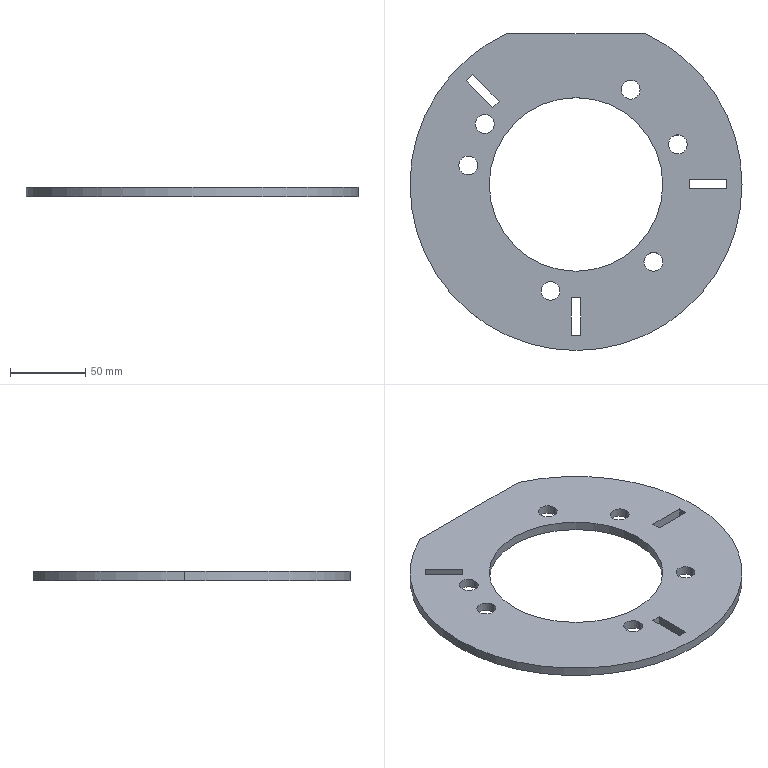Part | SolidWorks | features FlatPattern 1, SMBaseFlange 1, SheetMetal 1 | 1 solid | 32 faces | box 220 x 210 x 6 mm | volume 154940 mm3 | cylinder 17 | plane 15 | commonest cylinder face diameters 12.5 x12 220 x3 115 x2
STEP:
#1=CARTESIAN_POINT('',(92.731,46.962,6.));
#2=VERTEX_POINT('',#1);
#3=CARTESIAN_POINT('',(105.231,46.962,6.));
#4=VERTEX_POINT('',#3);
#5=CARTESIAN_POINT('',(98.981,46.962,6.));
#6=DIRECTION('',(0.,0.,1.));
#7=DIRECTION('',(1.,0.,0.));
#8=AXIS2_PLACEMENT_3D('',#5,#6,#7);
#9=CIRCLE('',#8,6.25);
#10=EDGE_CURVE('',#2,#4,#9,.T.);
#11=ORIENTED_EDGE('',*,*,#10,.T.);
#12=CARTESIAN_POINT('',(105.231,46.962,0.));
#13=VERTEX_POINT('',#12);
#14=CARTESIAN_POINT('',(105.231,46.962,6.));
#15=DIRECTION('',(0.,0.,-1.));
#16=VECTOR('',#15,1000.);
#17=LINE('',#14,#16);
#18=EDGE_CURVE('',#4,#13,#17,.T.);
#19=ORIENTED_EDGE('',*,*,#18,.T.);
#20=CARTESIAN_POINT('',(92.731,46.962,0.));
#21=VERTEX_POINT('',#20);
#22=CARTESIAN_POINT('',(98.981,46.962,0.));
#23=DIRECTION('',(0.,0.,1.));
#24=DIRECTION('',(1.,0.,0.));
#25=AXIS2_PLACEMENT_3D('',#22,#23,#24);
#26=CIRCLE('',#25,6.25);
#27=EDGE_CURVE('',#21,#13,#26,.T.);
#28=ORIENTED_EDGE('',*,*,#27,.F.);
#29=CARTESIAN_POINT('',(92.731,46.962,6.));
#30=DIRECTION('',(0.,0.,-1.));
#31=VECTOR('',#30,1000.);
#32=LINE('',#29,#31);
#33=EDGE_CURVE('',#2,#21,#32,.T.);
#34=ORIENTED_EDGE('',*,*,#33,.F.);
#35=EDGE_LOOP('',(#11,#19,#28,#34));
#36=FACE_OUTER_BOUND('',#35,.T.);
#37=CARTESIAN_POINT('',(98.981,46.962,6.));
#38=DIRECTION('',(0.,0.,-1.));
#39=DIRECTION('',(-1.,0.,0.));
#40=AXIS2_PLACEMENT_3D('',#37,#38,#39);
#41=CYLINDRICAL_SURFACE('',#40,6.25);
#42=ADVANCED_FACE('',(#36),#41,.F.);
#43=CARTESIAN_POINT('',(-3.976,24.191,6.));
#44=VERTEX_POINT('',#43);
#45=CARTESIAN_POINT('',(8.524,24.191,6.));
#46=VERTEX_POINT('',#45);
#47=CARTESIAN_POINT('',(2.274,24.191,6.));
#48=DIRECTION('',(0.,0.,1.));
#49=DIRECTION('',(1.,0.,0.));
#50=AXIS2_PLACEMENT_3D('',#47,#48,#49);
#51=CIRCLE('',#50,6.25);
#52=EDGE_CURVE('',#44,#46,#51,.T.);
#53=ORIENTED_EDGE('',*,*,#52,.T.);
#54=CARTESIAN_POINT('',(8.524,24.191,0.));
#55=VERTEX_POINT('',#54);
#56=CARTESIAN_POINT('',(8.524,24.191,6.));
#57=DIRECTION('',(0.,0.,-1.));
#58=VECTOR('',#57,1000.);
#59=LINE('',#56,#58);
#60=EDGE_CURVE('',#46,#55,#59,.T.);
#61=ORIENTED_EDGE('',*,*,#60,.T.);
#62=CARTESIAN_POINT('',(-3.976,24.191,0.));
#63=VERTEX_POINT('',#62);
#64=CARTESIAN_POINT('',(2.274,24.191,0.));
#65=DIRECTION('',(0.,0.,1.));
#66=DIRECTION('',(1.,0.,0.));
#67=AXIS2_PLACEMENT_3D('',#64,#65,#66);
#68=CIRCLE('',#67,6.25);
#69=EDGE_CURVE('',#63,#55,#68,.T.);
#70=ORIENTED_EDGE('',*,*,#69,.F.);
#71=CARTESIAN_POINT('',(-3.976,24.191,6.));
#72=DIRECTION('',(0.,0.,-1.));
#73=VECTOR('',#72,1000.);
#74=LINE('',#71,#73);
#75=EDGE_CURVE('',#44,#63,#74,.T.);
#76=ORIENTED_EDGE('',*,*,#75,.F.);
#77=EDGE_LOOP('',(#53,#61,#70,#76));
#78=FACE_OUTER_BOUND('',#77,.T.);
#79=CARTESIAN_POINT('',(2.274,24.191,6.));
#80=DIRECTION('',(0.,0.,-1.));
#81=DIRECTION('',(-1.,0.,0.));
#82=AXIS2_PLACEMENT_3D('',#79,#80,#81);
#83=CYLINDRICAL_SURFACE('',#82,6.25);
#84=ADVANCED_FACE('',(#78),#83,.F.);
#85=CARTESIAN_POINT('',(-14.918,-3.235,6.));
#86=VERTEX_POINT('',#85);
#87=CARTESIAN_POINT('',(-2.418,-3.235,6.));
#88=VERTEX_POINT('',#87);
#89=CARTESIAN_POINT('',(-8.668,-3.235,6.));
#90=DIRECTION('',(0.,0.,1.));
#91=DIRECTION('',(1.,0.,0.));
#92=AXIS2_PLACEMENT_3D('',#89,#90,#91);
#93=CIRCLE('',#92,6.25);
#94=EDGE_CURVE('',#86,#88,#93,.T.);
#95=ORIENTED_EDGE('',*,*,#94,.T.);
#96=CARTESIAN_POINT('',(-2.418,-3.235,0.));
#97=VERTEX_POINT('',#96);
#98=CARTESIAN_POINT('',(-2.418,-3.235,6.));
#99=DIRECTION('',(0.,0.,-1.));
#100=VECTOR('',#99,1000.);
#101=LINE('',#98,#100);
#102=EDGE_CURVE('',#88,#97,#101,.T.);
#103=ORIENTED_EDGE('',*,*,#102,.T.);
#104=CARTESIAN_POINT('',(-14.918,-3.235,0.));
#105=VERTEX_POINT('',#104);
#106=CARTESIAN_POINT('',(-8.668,-3.235,0.));
#107=DIRECTION('',(0.,0.,1.));
#108=DIRECTION('',(1.,0.,0.));
#109=AXIS2_PLACEMENT_3D('',#106,#107,#108);
#110=CIRCLE('',#109,6.25);
#111=EDGE_CURVE('',#105,#97,#110,.T.);
#112=ORIENTED_EDGE('',*,*,#111,.F.);
#113=CARTESIAN_POINT('',(-14.918,-3.235,6.));
#114=DIRECTION('',(0.,0.,-1.));
#115=VECTOR('',#114,1000.);
#116=LINE('',#113,#115);
#117=EDGE_CURVE('',#86,#105,#116,.T.);
#118=ORIENTED_EDGE('',*,*,#117,.F.);
#119=EDGE_LOOP('',(#95,#103,#112,#118));
#120=FACE_OUTER_BOUND('',#119,.T.);
#121=CARTESIAN_POINT('',(-8.668,-3.235,6.));
#122=DIRECTION('',(0.,0.,-1.));
#123=DIRECTION('',(-1.,0.,0.));
#124=AXIS2_PLACEMENT_3D('',#121,#122,#123);
#125=CYLINDRICAL_SURFACE('',#124,6.25);
#126=ADVANCED_FACE('',(#120),#125,.F.);
#127=CARTESIAN_POINT('',(39.556,-86.321,6.));
#128=VERTEX_POINT('',#127);
#129=CARTESIAN_POINT('',(52.056,-86.321,6.));
#130=VERTEX_POINT('',#129);
#131=CARTESIAN_POINT('',(45.806,-86.321,6.));
#132=DIRECTION('',(0.,0.,1.));
#133=DIRECTION('',(1.,0.,0.));
#134=AXIS2_PLACEMENT_3D('',#131,#132,#133);
#135=CIRCLE('',#134,6.25);
#136=EDGE_CURVE('',#128,#130,#135,.T.);
#137=ORIENTED_EDGE('',*,*,#136,.T.);
#138=CARTESIAN_POINT('',(52.056,-86.321,0.));
#139=VERTEX_POINT('',#138);
#140=CARTESIAN_POINT('',(52.056,-86.321,6.));
#141=DIRECTION('',(0.,0.,-1.));
#142=VECTOR('',#141,1000.);
#143=LINE('',#140,#142);
#144=EDGE_CURVE('',#130,#139,#143,.T.);
#145=ORIENTED_EDGE('',*,*,#144,.T.);
#146=CARTESIAN_POINT('',(39.556,-86.321,0.));
#147=VERTEX_POINT('',#146);
#148=CARTESIAN_POINT('',(45.806,-86.321,0.));
#149=DIRECTION('',(0.,0.,1.));
#150=DIRECTION('',(1.,0.,0.));
#151=AXIS2_PLACEMENT_3D('',#148,#149,#150);
#152=CIRCLE('',#151,6.25);
#153=EDGE_CURVE('',#147,#139,#152,.T.);
#154=ORIENTED_EDGE('',*,*,#153,.F.);
#155=CARTESIAN_POINT('',(39.556,-86.321,6.));
#156=DIRECTION('',(0.,0.,-1.));
#157=VECTOR('',#156,1000.);
#158=LINE('',#155,#157);
#159=EDGE_CURVE('',#128,#147,#158,.T.);
#160=ORIENTED_EDGE('',*,*,#159,.F.);
#161=EDGE_LOOP('',(#137,#145,#154,#160));
#162=FACE_OUTER_BOUND('',#161,.T.);
#163=CARTESIAN_POINT('',(45.806,-86.321,6.));
#164=DIRECTION('',(0.,0.,-1.));
#165=DIRECTION('',(-1.,0.,0.));
#166=AXIS2_PLACEMENT_3D('',#163,#164,#165);
#167=CYLINDRICAL_SURFACE('',#166,6.25);
#168=ADVANCED_FACE('',(#162),#167,.F.);
#169=CARTESIAN_POINT('',(107.746,-67.09,6.));
#170=VERTEX_POINT('',#169);
#171=CARTESIAN_POINT('',(120.246,-67.09,6.));
#172=VERTEX_POINT('',#171);
#173=CARTESIAN_POINT('',(113.996,-67.09,6.));
#174=DIRECTION('',(0.,0.,1.));
#175=DIRECTION('',(1.,0.,0.));
#176=AXIS2_PLACEMENT_3D('',#173,#174,#175);
#177=CIRCLE('',#176,6.25);
#178=EDGE_CURVE('',#170,#172,#177,.T.);
#179=ORIENTED_EDGE('',*,*,#178,.T.);
#180=CARTESIAN_POINT('',(120.246,-67.09,0.));
#181=VERTEX_POINT('',#180);
#182=CARTESIAN_POINT('',(120.246,-67.09,6.));
#183=DIRECTION('',(0.,0.,-1.));
#184=VECTOR('',#183,1000.);
#185=LINE('',#182,#184);
#186=EDGE_CURVE('',#172,#181,#185,.T.);
#187=ORIENTED_EDGE('',*,*,#186,.T.);
#188=CARTESIAN_POINT('',(107.746,-67.09,0.));
#189=VERTEX_POINT('',#188);
#190=CARTESIAN_POINT('',(113.996,-67.09,0.));
#191=DIRECTION('',(0.,0.,1.));
#192=DIRECTION('',(1.,0.,0.));
#193=AXIS2_PLACEMENT_3D('',#190,#191,#192);
#194=CIRCLE('',#193,6.25);
#195=EDGE_CURVE('',#189,#181,#194,.T.);
#196=ORIENTED_EDGE('',*,*,#195,.F.);
#197=CARTESIAN_POINT('',(107.746,-67.09,6.));
#198=DIRECTION('',(0.,0.,-1.));
#199=VECTOR('',#198,1000.);
#200=LINE('',#197,#199);
#201=EDGE_CURVE('',#170,#189,#200,.T.);
#202=ORIENTED_EDGE('',*,*,#201,.F.);
#203=EDGE_LOOP('',(#179,#187,#196,#202));
#204=FACE_OUTER_BOUND('',#203,.T.);
#205=CARTESIAN_POINT('',(113.996,-67.09,6.));
#206=DIRECTION('',(0.,0.,-1.));
#207=DIRECTION('',(-1.,0.,0.));
#208=AXIS2_PLACEMENT_3D('',#205,#206,#207);
#209=CYLINDRICAL_SURFACE('',#208,6.25);
#210=ADVANCED_FACE('',(#204),#209,.F.);
#211=CARTESIAN_POINT('',(123.936,10.747,6.));
#212=VERTEX_POINT('',#211);
#213=CARTESIAN_POINT('',(136.436,10.747,6.));
#214=VERTEX_POINT('',#213);
#215=CARTESIAN_POINT('',(130.186,10.747,6.));
#216=DIRECTION('',(0.,0.,1.));
#217=DIRECTION('',(1.,0.,0.));
#218=AXIS2_PLACEMENT_3D('',#215,#216,#217);
#219=CIRCLE('',#218,6.25);
#220=EDGE_CURVE('',#212,#214,#219,.T.);
#221=ORIENTED_EDGE('',*,*,#220,.T.);
#222=CARTESIAN_POINT('',(136.436,10.747,0.));
#223=VERTEX_POINT('',#222);
#224=CARTESIAN_POINT('',(136.436,10.747,6.));
#225=DIRECTION('',(0.,0.,-1.));
#226=VECTOR('',#225,1000.);
#227=LINE('',#224,#226);
#228=EDGE_CURVE('',#214,#223,#227,.T.);
#229=ORIENTED_EDGE('',*,*,#228,.T.);
#230=CARTESIAN_POINT('',(123.936,10.747,0.));
#231=VERTEX_POINT('',#230);
#232=CARTESIAN_POINT('',(130.186,10.747,0.));
#233=DIRECTION('',(0.,0.,1.));
#234=DIRECTION('',(1.,0.,0.));
#235=AXIS2_PLACEMENT_3D('',#232,#233,#234);
#236=CIRCLE('',#235,6.25);
#237=EDGE_CURVE('',#231,#223,#236,.T.);
#238=ORIENTED_EDGE('',*,*,#237,.F.);
#239=CARTESIAN_POINT('',(123.936,10.747,6.));
#240=DIRECTION('',(0.,0.,-1.));
#241=VECTOR('',#240,1000.);
#242=LINE('',#239,#241);
#243=EDGE_CURVE('',#212,#231,#242,.T.);
#244=ORIENTED_EDGE('',*,*,#243,.F.);
#245=EDGE_LOOP('',(#221,#229,#238,#244));
#246=FACE_OUTER_BOUND('',#245,.T.);
#247=CARTESIAN_POINT('',(130.186,10.747,6.));
#248=DIRECTION('',(0.,0.,-1.));
#249=DIRECTION('',(-1.,0.,0.));
#250=AXIS2_PLACEMENT_3D('',#247,#248,#249);
#251=CYLINDRICAL_SURFACE('',#250,6.25);
#252=ADVANCED_FACE('',(#246),#251,.F.);
#253=CARTESIAN_POINT('',(5.231,-15.825,6.));
#254=VERTEX_POINT('',#253);
#255=CARTESIAN_POINT('',(120.231,-15.825,6.));
#256=VERTEX_POINT('',#255);
#257=CARTESIAN_POINT('',(62.731,-15.825,6.));
#258=DIRECTION('',(0.,0.,1.));
#259=DIRECTION('',(1.,0.,0.));
#260=AXIS2_PLACEMENT_3D('',#257,#258,#259);
#261=CIRCLE('',#260,57.5);
#262=EDGE_CURVE('',#254,#256,#261,.T.);
#263=ORIENTED_EDGE('',*,*,#262,.T.);
#264=CARTESIAN_POINT('',(120.231,-15.825,0.));
#265=VERTEX_POINT('',#264);
#266=CARTESIAN_POINT('',(120.231,-15.825,6.));
#267=DIRECTION('',(0.,0.,-1.));
#268=VECTOR('',#267,1000.);
#269=LINE('',#266,#268);
#270=EDGE_CURVE('',#256,#265,#269,.T.);
#271=ORIENTED_EDGE('',*,*,#270,.T.);
#272=CARTESIAN_POINT('',(5.231,-15.825,0.));
#273=VERTEX_POINT('',#272);
#274=CARTESIAN_POINT('',(62.731,-15.825,0.));
#275=DIRECTION('',(0.,0.,1.));
#276=DIRECTION('',(1.,0.,0.));
#277=AXIS2_PLACEMENT_3D('',#274,#275,#276);
#278=CIRCLE('',#277,57.5);
#279=EDGE_CURVE('',#273,#265,#278,.T.);
#280=ORIENTED_EDGE('',*,*,#279,.F.);
#281=CARTESIAN_POINT('',(5.231,-15.825,6.));
#282=DIRECTION('',(0.,0.,-1.));
#283=VECTOR('',#282,1000.);
#284=LINE('',#281,#283);
#285=EDGE_CURVE('',#254,#273,#284,.T.);
#286=ORIENTED_EDGE('',*,*,#285,.F.);
#287=EDGE_LOOP('',(#263,#271,#280,#286));
#288=FACE_OUTER_BOUND('',#287,.T.);
#289=CARTESIAN_POINT('',(62.731,-15.825,6.));
#290=DIRECTION('',(0.,0.,-1.));
#291=DIRECTION('',(-1.,0.,0.));
#292=AXIS2_PLACEMENT_3D('',#289,#290,#291);
#293=CYLINDRICAL_SURFACE('',#292,57.5);
#294=ADVANCED_FACE('',(#288),#293,.F.);
#295=CARTESIAN_POINT('',(172.731,-15.825,6.));
#296=VERTEX_POINT('',#295);
#297=CARTESIAN_POINT('',(108.557,84.175,6.));
#298=VERTEX_POINT('',#297);
#299=CARTESIAN_POINT('',(62.731,-15.825,6.));
#300=DIRECTION('',(0.,0.,1.));
#301=DIRECTION('',(1.,0.,0.));
#302=AXIS2_PLACEMENT_3D('',#299,#300,#301);
#303=CIRCLE('',#302,110.);
#304=EDGE_CURVE('',#296,#298,#303,.T.);
#305=ORIENTED_EDGE('',*,*,#304,.F.);
#306=CARTESIAN_POINT('',(172.731,-15.825,0.));
#307=VERTEX_POINT('',#306);
#308=CARTESIAN_POINT('',(172.731,-15.825,6.));
#309=DIRECTION('',(0.,0.,-1.));
#310=VECTOR('',#309,1000.);
#311=LINE('',#308,#310);
#312=EDGE_CURVE('',#296,#307,#311,.T.);
#313=ORIENTED_EDGE('',*,*,#312,.T.);
#314=CARTESIAN_POINT('',(108.557,84.175,0.));
#315=VERTEX_POINT('',#314);
#316=CARTESIAN_POINT('',(62.731,-15.825,0.));
#317=DIRECTION('',(0.,0.,1.));
#318=DIRECTION('',(1.,0.,0.));
#319=AXIS2_PLACEMENT_3D('',#316,#317,#318);
#320=CIRCLE('',#319,110.);
#321=EDGE_CURVE('',#307,#315,#320,.T.);
#322=ORIENTED_EDGE('',*,*,#321,.T.);
#323=CARTESIAN_POINT('',(108.557,84.175,6.));
#324=DIRECTION('',(0.,0.,-1.));
#325=VECTOR('',#324,1000.);
#326=LINE('',#323,#325);
#327=EDGE_CURVE('',#298,#315,#326,.T.);
#328=ORIENTED_EDGE('',*,*,#327,.F.);
#329=EDGE_LOOP('',(#305,#313,#322,#328));
#330=FACE_OUTER_BOUND('',#329,.T.);
#331=CARTESIAN_POINT('',(62.731,-15.825,6.));
#332=DIRECTION('',(0.,0.,-1.));
#333=DIRECTION('',(-1.,0.,0.));
#334=AXIS2_PLACEMENT_3D('',#331,#332,#333);
#335=CYLINDRICAL_SURFACE('',#334,110.);
#336=ADVANCED_FACE('',(#330),#335,.T.);
#337=ORIENTED_EDGE('',*,*,#312,.F.);
#338=CARTESIAN_POINT('',(-47.269,-15.825,6.));
#339=VERTEX_POINT('',#338);
#340=CARTESIAN_POINT('',(62.731,-15.825,6.));
#341=DIRECTION('',(0.,0.,1.));
#342=DIRECTION('',(1.,0.,0.));
#343=AXIS2_PLACEMENT_3D('',#340,#341,#342);
#344=CIRCLE('',#343,110.);
#345=EDGE_CURVE('',#339,#296,#344,.T.);
#346=ORIENTED_EDGE('',*,*,#345,.F.);
#347=CARTESIAN_POINT('',(-47.269,-15.825,0.));
#348=VERTEX_POINT('',#347);
#349=CARTESIAN_POINT('',(-47.269,-15.825,6.));
#350=DIRECTION('',(0.,0.,-1.));
#351=VECTOR('',#350,1000.);
#352=LINE('',#349,#351);
#353=EDGE_CURVE('',#339,#348,#352,.T.);
#354=ORIENTED_EDGE('',*,*,#353,.T.);
#355=CARTESIAN_POINT('',(62.731,-15.825,0.));
#356=DIRECTION('',(0.,0.,1.));
#357=DIRECTION('',(1.,0.,0.));
#358=AXIS2_PLACEMENT_3D('',#355,#356,#357);
#359=CIRCLE('',#358,110.);
#360=EDGE_CURVE('',#348,#307,#359,.T.);
#361=ORIENTED_EDGE('',*,*,#360,.T.);
#362=EDGE_LOOP('',(#337,#346,#354,#361));
#363=FACE_OUTER_BOUND('',#362,.T.);
#364=CARTESIAN_POINT('',(62.731,-15.825,6.));
#365=DIRECTION('',(0.,0.,-1.));
#366=DIRECTION('',(-1.,0.,0.));
#367=AXIS2_PLACEMENT_3D('',#364,#365,#366);
#368=CYLINDRICAL_SURFACE('',#367,110.);
#369=ADVANCED_FACE('',(#363),#368,.T.);
#370=ORIENTED_EDGE('',*,*,#52,.F.);
#371=CARTESIAN_POINT('',(2.274,24.191,6.));
#372=DIRECTION('',(0.,0.,1.));
#373=DIRECTION('',(1.,0.,0.));
#374=AXIS2_PLACEMENT_3D('',#371,#372,#373);
#375=CIRCLE('',#374,6.25);
#376=EDGE_CURVE('',#46,#44,#375,.T.);
#377=ORIENTED_EDGE('',*,*,#376,.F.);
#378=EDGE_LOOP('',(#370,#377));
#379=FACE_BOUND('',#378,.T.);
#380=ORIENTED_EDGE('',*,*,#136,.F.);
#381=CARTESIAN_POINT('',(45.806,-86.321,6.));
#382=DIRECTION('',(0.,0.,1.));
#383=DIRECTION('',(1.,0.,0.));
#384=AXIS2_PLACEMENT_3D('',#381,#382,#383);
#385=CIRCLE('',#384,6.25);
#386=EDGE_CURVE('',#130,#128,#385,.T.);
#387=ORIENTED_EDGE('',*,*,#386,.F.);
#388=EDGE_LOOP('',(#380,#387));
#389=FACE_BOUND('',#388,.T.);
#390=ORIENTED_EDGE('',*,*,#220,.F.);
#391=CARTESIAN_POINT('',(130.186,10.747,6.));
#392=DIRECTION('',(0.,0.,1.));
#393=DIRECTION('',(1.,0.,0.));
#394=AXIS2_PLACEMENT_3D('',#391,#392,#393);
#395=CIRCLE('',#394,6.25);
#396=EDGE_CURVE('',#214,#212,#395,.T.);
#397=ORIENTED_EDGE('',*,*,#396,.F.);
#398=EDGE_LOOP('',(#390,#397));
#399=FACE_BOUND('',#398,.T.);
#400=CARTESIAN_POINT('',(16.905,84.175,6.));
#401=VERTEX_POINT('',#400);
#402=CARTESIAN_POINT('',(62.731,-15.825,6.));
#403=DIRECTION('',(0.,0.,1.));
#404=DIRECTION('',(1.,0.,0.));
#405=AXIS2_PLACEMENT_3D('',#402,#403,#404);
#406=CIRCLE('',#405,110.);
#407=EDGE_CURVE('',#401,#339,#406,.T.);
#408=ORIENTED_EDGE('',*,*,#407,.T.);
#409=ORIENTED_EDGE('',*,*,#345,.T.);
#410=ORIENTED_EDGE('',*,*,#304,.T.);
#411=CARTESIAN_POINT('',(16.905,84.175,6.));
#412=DIRECTION('',(-1.,0.,0.));
#413=VECTOR('',#412,1000.);
#414=LINE('',#411,#413);
#415=EDGE_CURVE('',#298,#401,#414,.T.);
#416=ORIENTED_EDGE('',*,*,#415,.T.);
#417=EDGE_LOOP('',(#408,#409,#410,#416));
#418=FACE_OUTER_BOUND('',#417,.T.);
#419=ORIENTED_EDGE('',*,*,#262,.F.);
#420=CARTESIAN_POINT('',(62.731,-15.825,6.));
#421=DIRECTION('',(0.,0.,1.));
#422=DIRECTION('',(1.,0.,0.));
#423=AXIS2_PLACEMENT_3D('',#420,#421,#422);
#424=CIRCLE('',#423,57.5);
#425=EDGE_CURVE('',#256,#254,#424,.T.);
#426=ORIENTED_EDGE('',*,*,#425,.F.);
#427=EDGE_LOOP('',(#419,#426));
#428=FACE_BOUND('',#427,.T.);
#429=ORIENTED_EDGE('',*,*,#178,.F.);
#430=CARTESIAN_POINT('',(113.996,-67.09,6.));
#431=DIRECTION('',(0.,0.,1.));
#432=DIRECTION('',(1.,0.,0.));
#433=AXIS2_PLACEMENT_3D('',#430,#431,#432);
#434=CIRCLE('',#433,6.25);
#435=EDGE_CURVE('',#172,#170,#434,.T.);
#436=ORIENTED_EDGE('',*,*,#435,.F.);
#437=EDGE_LOOP('',(#429,#436));
#438=FACE_BOUND('',#437,.T.);
#439=ORIENTED_EDGE('',*,*,#94,.F.);
#440=CARTESIAN_POINT('',(-8.668,-3.235,6.));
#441=DIRECTION('',(0.,0.,1.));
#442=DIRECTION('',(1.,0.,0.));
#443=AXIS2_PLACEMENT_3D('',#440,#441,#442);
#444=CIRCLE('',#443,6.25);
#445=EDGE_CURVE('',#88,#86,#444,.T.);
#446=ORIENTED_EDGE('',*,*,#445,.F.);
#447=EDGE_LOOP('',(#439,#446));
#448=FACE_BOUND('',#447,.T.);
#449=ORIENTED_EDGE('',*,*,#10,.F.);
#450=CARTESIAN_POINT('',(98.981,46.962,6.));
#451=DIRECTION('',(0.,0.,1.));
#452=DIRECTION('',(1.,0.,0.));
#453=AXIS2_PLACEMENT_3D('',#450,#451,#452);
#454=CIRCLE('',#453,6.25);
#455=EDGE_CURVE('',#4,#2,#454,.T.);
#456=ORIENTED_EDGE('',*,*,#455,.F.);
#457=EDGE_LOOP('',(#449,#456));
#458=FACE_BOUND('',#457,.T.);
#459=CARTESIAN_POINT('',(162.731,-12.825,6.));
#460=VERTEX_POINT('',#459);
#461=CARTESIAN_POINT('',(137.731,-12.825,6.));
#462=VERTEX_POINT('',#461);
#463=CARTESIAN_POINT('',(162.731,-12.825,6.));
#464=DIRECTION('',(-1.,0.,0.));
#465=VECTOR('',#464,1000.);
#466=LINE('',#463,#465);
#467=EDGE_CURVE('',#460,#462,#466,.T.);
#468=ORIENTED_EDGE('',*,*,#467,.F.);
#469=CARTESIAN_POINT('',(162.731,-18.825,6.));
#470=VERTEX_POINT('',#469);
#471=CARTESIAN_POINT('',(162.731,-18.825,6.));
#472=DIRECTION('',(0.,1.,0.));
#473=VECTOR('',#472,1000.);
#474=LINE('',#471,#473);
#475=EDGE_CURVE('',#470,#460,#474,.T.);
#476=ORIENTED_EDGE('',*,*,#475,.F.);
#477=CARTESIAN_POINT('',(137.731,-18.825,6.));
#478=VERTEX_POINT('',#477);
#479=CARTESIAN_POINT('',(137.731,-18.825,6.));
#480=DIRECTION('',(1.,0.,0.));
#481=VECTOR('',#480,1000.);
#482=LINE('',#479,#481);
#483=EDGE_CURVE('',#478,#470,#482,.T.);
#484=ORIENTED_EDGE('',*,*,#483,.F.);
#485=CARTESIAN_POINT('',(137.731,-12.825,6.));
#486=DIRECTION('',(0.,-1.,0.));
#487=VECTOR('',#486,1000.);
#488=LINE('',#485,#487);
#489=EDGE_CURVE('',#462,#478,#488,.T.);
#490=ORIENTED_EDGE('',*,*,#489,.F.);
#491=EDGE_LOOP('',(#468,#476,#484,#490));
#492=FACE_BOUND('',#491,.T.);
#493=CARTESIAN_POINT('',(-10.101,52.765,6.));
#494=VERTEX_POINT('',#493);
#495=CARTESIAN_POINT('',(7.577,35.087,6.));
#496=VERTEX_POINT('',#495);
#497=CARTESIAN_POINT('',(7.577,35.087,6.));
#498=DIRECTION('',(0.7071,-0.7071,0.));
#499=VECTOR('',#498,1000.);
#500=LINE('',#497,#499);
#501=EDGE_CURVE('',#494,#496,#500,.T.);
#502=ORIENTED_EDGE('',*,*,#501,.F.);
#503=CARTESIAN_POINT('',(-5.858,57.007,6.));
#504=VERTEX_POINT('',#503);
#505=CARTESIAN_POINT('',(-10.101,52.765,6.));
#506=DIRECTION('',(-0.7071,-0.7071,0.));
#507=VECTOR('',#506,1000.);
#508=LINE('',#505,#507);
#509=EDGE_CURVE('',#504,#494,#508,.T.);
#510=ORIENTED_EDGE('',*,*,#509,.F.);
#511=CARTESIAN_POINT('',(11.819,39.33,6.));
#512=VERTEX_POINT('',#511);
#513=CARTESIAN_POINT('',(-5.858,57.007,6.));
#514=DIRECTION('',(-0.7071,0.7071,0.));
#515=VECTOR('',#514,1000.);
#516=LINE('',#513,#515);
#517=EDGE_CURVE('',#512,#504,#516,.T.);
#518=ORIENTED_EDGE('',*,*,#517,.F.);
#519=CARTESIAN_POINT('',(11.819,39.33,6.));
#520=DIRECTION('',(0.7071,0.7071,0.));
#521=VECTOR('',#520,1000.);
#522=LINE('',#519,#521);
#523=EDGE_CURVE('',#496,#512,#522,.T.);
#524=ORIENTED_EDGE('',*,*,#523,.F.);
#525=EDGE_LOOP('',(#502,#510,#518,#524));
#526=FACE_BOUND('',#525,.T.);
#527=CARTESIAN_POINT('',(65.731,-90.825,6.));
#528=VERTEX_POINT('',#527);
#529=CARTESIAN_POINT('',(59.731,-90.825,6.));
#530=VERTEX_POINT('',#529);
#531=CARTESIAN_POINT('',(65.731,-90.825,6.));
#532=DIRECTION('',(-1.,0.,0.));
#533=VECTOR('',#532,1000.);
#534=LINE('',#531,#533);
#535=EDGE_CURVE('',#528,#530,#534,.T.);
#536=ORIENTED_EDGE('',*,*,#535,.F.);
#537=CARTESIAN_POINT('',(65.731,-115.825,6.));
#538=VERTEX_POINT('',#537);
#539=CARTESIAN_POINT('',(65.731,-115.825,6.));
#540=DIRECTION('',(0.,1.,0.));
#541=VECTOR('',#540,1000.);
#542=LINE('',#539,#541);
#543=EDGE_CURVE('',#538,#528,#542,.T.);
#544=ORIENTED_EDGE('',*,*,#543,.F.);
#545=CARTESIAN_POINT('',(59.731,-115.825,6.));
#546=VERTEX_POINT('',#545);
#547=CARTESIAN_POINT('',(59.731,-115.825,6.));
#548=DIRECTION('',(1.,0.,0.));
#549=VECTOR('',#548,1000.);
#550=LINE('',#547,#549);
#551=EDGE_CURVE('',#546,#538,#550,.T.);
#552=ORIENTED_EDGE('',*,*,#551,.F.);
#553=CARTESIAN_POINT('',(59.731,-90.825,6.));
#554=DIRECTION('',(0.,-1.,0.));
#555=VECTOR('',#554,1000.);
#556=LINE('',#553,#555);
#557=EDGE_CURVE('',#530,#546,#556,.T.);
#558=ORIENTED_EDGE('',*,*,#557,.F.);
#559=EDGE_LOOP('',(#536,#544,#552,#558));
#560=FACE_BOUND('',#559,.T.);
#561=CARTESIAN_POINT('',(62.731,-15.825,6.));
#562=DIRECTION('',(0.,0.,1.));
#563=DIRECTION('',(1.,0.,0.));
#564=AXIS2_PLACEMENT_3D('',#561,#562,#563);
#565=PLANE('',#564);
#566=ADVANCED_FACE('',(#379,#389,#399,#418,#428,#438,#448,#458,#492,#526,#560),#565,.T.);
#567=CARTESIAN_POINT('',(-5.858,57.007,0.));
#568=VERTEX_POINT('',#567);
#569=CARTESIAN_POINT('',(-10.101,52.765,0.));
#570=VERTEX_POINT('',#569);
#571=CARTESIAN_POINT('',(-10.101,52.765,0.));
#572=DIRECTION('',(-0.7071,-0.7071,0.));
#573=VECTOR('',#572,1000.);
#574=LINE('',#571,#573);
#575=EDGE_CURVE('',#568,#570,#574,.T.);
#576=ORIENTED_EDGE('',*,*,#575,.T.);
#577=CARTESIAN_POINT('',(7.577,35.087,0.));
#578=VERTEX_POINT('',#577);
#579=CARTESIAN_POINT('',(7.577,35.087,0.));
#580=DIRECTION('',(0.7071,-0.7071,0.));
#581=VECTOR('',#580,1000.);
#582=LINE('',#579,#581);
#583=EDGE_CURVE('',#570,#578,#582,.T.);
#584=ORIENTED_EDGE('',*,*,#583,.T.);
#585=CARTESIAN_POINT('',(11.819,39.33,0.));
#586=VERTEX_POINT('',#585);
#587=CARTESIAN_POINT('',(11.819,39.33,0.));
#588=DIRECTION('',(0.7071,0.7071,0.));
#589=VECTOR('',#588,1000.);
#590=LINE('',#587,#589);
#591=EDGE_CURVE('',#578,#586,#590,.T.);
#592=ORIENTED_EDGE('',*,*,#591,.T.);
#593=CARTESIAN_POINT('',(-5.858,57.007,0.));
#594=DIRECTION('',(-0.7071,0.7071,0.));
#595=VECTOR('',#594,1000.);
#596=LINE('',#593,#595);
#597=EDGE_CURVE('',#586,#568,#596,.T.);
#598=ORIENTED_EDGE('',*,*,#597,.T.);
#599=EDGE_LOOP('',(#576,#584,#592,#598));
#600=FACE_BOUND('',#599,.T.);
#601=ORIENTED_EDGE('',*,*,#27,.T.);
#602=CARTESIAN_POINT('',(98.981,46.962,0.));
#603=DIRECTION('',(0.,0.,1.));
#604=DIRECTION('',(1.,0.,0.));
#605=AXIS2_PLACEMENT_3D('',#602,#603,#604);
#606=CIRCLE('',#605,6.25);
#607=EDGE_CURVE('',#13,#21,#606,.T.);
#608=ORIENTED_EDGE('',*,*,#607,.T.);
#609=EDGE_LOOP('',(#601,#608));
#610=FACE_BOUND('',#609,.T.);
#611=ORIENTED_EDGE('',*,*,#69,.T.);
#612=CARTESIAN_POINT('',(2.274,24.191,0.));
#613=DIRECTION('',(0.,0.,1.));
#614=DIRECTION('',(1.,0.,0.));
#615=AXIS2_PLACEMENT_3D('',#612,#613,#614);
#616=CIRCLE('',#615,6.25);
#617=EDGE_CURVE('',#55,#63,#616,.T.);
#618=ORIENTED_EDGE('',*,*,#617,.T.);
#619=EDGE_LOOP('',(#611,#618));
#620=FACE_BOUND('',#619,.T.);
#621=ORIENTED_EDGE('',*,*,#111,.T.);
#622=CARTESIAN_POINT('',(-8.668,-3.235,0.));
#623=DIRECTION('',(0.,0.,1.));
#624=DIRECTION('',(1.,0.,0.));
#625=AXIS2_PLACEMENT_3D('',#622,#623,#624);
#626=CIRCLE('',#625,6.25);
#627=EDGE_CURVE('',#97,#105,#626,.T.);
#628=ORIENTED_EDGE('',*,*,#627,.T.);
#629=EDGE_LOOP('',(#621,#628));
#630=FACE_BOUND('',#629,.T.);
#631=ORIENTED_EDGE('',*,*,#153,.T.);
#632=CARTESIAN_POINT('',(45.806,-86.321,0.));
#633=DIRECTION('',(0.,0.,1.));
#634=DIRECTION('',(1.,0.,0.));
#635=AXIS2_PLACEMENT_3D('',#632,#633,#634);
#636=CIRCLE('',#635,6.25);
#637=EDGE_CURVE('',#139,#147,#636,.T.);
#638=ORIENTED_EDGE('',*,*,#637,.T.);
#639=EDGE_LOOP('',(#631,#638));
#640=FACE_BOUND('',#639,.T.);
#641=ORIENTED_EDGE('',*,*,#195,.T.);
#642=CARTESIAN_POINT('',(113.996,-67.09,0.));
#643=DIRECTION('',(0.,0.,1.));
#644=DIRECTION('',(1.,0.,0.));
#645=AXIS2_PLACEMENT_3D('',#642,#643,#644);
#646=CIRCLE('',#645,6.25);
#647=EDGE_CURVE('',#181,#189,#646,.T.);
#648=ORIENTED_EDGE('',*,*,#647,.T.);
#649=EDGE_LOOP('',(#641,#648));
#650=FACE_BOUND('',#649,.T.);
#651=ORIENTED_EDGE('',*,*,#237,.T.);
#652=CARTESIAN_POINT('',(130.186,10.747,0.));
#653=DIRECTION('',(0.,0.,1.));
#654=DIRECTION('',(1.,0.,0.));
#655=AXIS2_PLACEMENT_3D('',#652,#653,#654);
#656=CIRCLE('',#655,6.25);
#657=EDGE_CURVE('',#223,#231,#656,.T.);
#658=ORIENTED_EDGE('',*,*,#657,.T.);
#659=EDGE_LOOP('',(#651,#658));
#660=FACE_BOUND('',#659,.T.);
#661=ORIENTED_EDGE('',*,*,#279,.T.);
#662=CARTESIAN_POINT('',(62.731,-15.825,0.));
#663=DIRECTION('',(0.,0.,1.));
#664=DIRECTION('',(1.,0.,0.));
#665=AXIS2_PLACEMENT_3D('',#662,#663,#664);
#666=CIRCLE('',#665,57.5);
#667=EDGE_CURVE('',#265,#273,#666,.T.);
#668=ORIENTED_EDGE('',*,*,#667,.T.);
#669=EDGE_LOOP('',(#661,#668));
#670=FACE_BOUND('',#669,.T.);
#671=CARTESIAN_POINT('',(16.905,84.175,0.));
#672=VERTEX_POINT('',#671);
#673=CARTESIAN_POINT('',(62.731,-15.825,0.));
#674=DIRECTION('',(0.,0.,1.));
#675=DIRECTION('',(1.,0.,0.));
#676=AXIS2_PLACEMENT_3D('',#673,#674,#675);
#677=CIRCLE('',#676,110.);
#678=EDGE_CURVE('',#672,#348,#677,.T.);
#679=ORIENTED_EDGE('',*,*,#678,.F.);
#680=CARTESIAN_POINT('',(16.905,84.175,0.));
#681=DIRECTION('',(-1.,0.,0.));
#682=VECTOR('',#681,1000.);
#683=LINE('',#680,#682);
#684=EDGE_CURVE('',#315,#672,#683,.T.);
#685=ORIENTED_EDGE('',*,*,#684,.F.);
#686=ORIENTED_EDGE('',*,*,#321,.F.);
#687=ORIENTED_EDGE('',*,*,#360,.F.);
#688=EDGE_LOOP('',(#679,#685,#686,#687));
#689=FACE_OUTER_BOUND('',#688,.T.);
#690=CARTESIAN_POINT('',(162.731,-18.825,0.));
#691=VERTEX_POINT('',#690);
#692=CARTESIAN_POINT('',(162.731,-12.825,0.));
#693=VERTEX_POINT('',#692);
#694=CARTESIAN_POINT('',(162.731,-18.825,0.));
#695=DIRECTION('',(0.,1.,0.));
#696=VECTOR('',#695,1000.);
#697=LINE('',#694,#696);
#698=EDGE_CURVE('',#691,#693,#697,.T.);
#699=ORIENTED_EDGE('',*,*,#698,.T.);
#700=CARTESIAN_POINT('',(137.731,-12.825,0.));
#701=VERTEX_POINT('',#700);
#702=CARTESIAN_POINT('',(162.731,-12.825,0.));
#703=DIRECTION('',(-1.,0.,0.));
#704=VECTOR('',#703,1000.);
#705=LINE('',#702,#704);
#706=EDGE_CURVE('',#693,#701,#705,.T.);
#707=ORIENTED_EDGE('',*,*,#706,.T.);
#708=CARTESIAN_POINT('',(137.731,-18.825,0.));
#709=VERTEX_POINT('',#708);
#710=CARTESIAN_POINT('',(137.731,-12.825,0.));
#711=DIRECTION('',(0.,-1.,0.));
#712=VECTOR('',#711,1000.);
#713=LINE('',#710,#712);
#714=EDGE_CURVE('',#701,#709,#713,.T.);
#715=ORIENTED_EDGE('',*,*,#714,.T.);
#716=CARTESIAN_POINT('',(137.731,-18.825,0.));
#717=DIRECTION('',(1.,0.,0.));
#718=VECTOR('',#717,1000.);
#719=LINE('',#716,#718);
#720=EDGE_CURVE('',#709,#691,#719,.T.);
#721=ORIENTED_EDGE('',*,*,#720,.T.);
#722=EDGE_LOOP('',(#699,#707,#715,#721));
#723=FACE_BOUND('',#722,.T.);
#724=CARTESIAN_POINT('',(65.731,-115.825,0.));
#725=VERTEX_POINT('',#724);
#726=CARTESIAN_POINT('',(65.731,-90.825,0.));
#727=VERTEX_POINT('',#726);
#728=CARTESIAN_POINT('',(65.731,-115.825,0.));
#729=DIRECTION('',(0.,1.,0.));
#730=VECTOR('',#729,1000.);
#731=LINE('',#728,#730);
#732=EDGE_CURVE('',#725,#727,#731,.T.);
#733=ORIENTED_EDGE('',*,*,#732,.T.);
#734=CARTESIAN_POINT('',(59.731,-90.825,0.));
#735=VERTEX_POINT('',#734);
#736=CARTESIAN_POINT('',(65.731,-90.825,0.));
#737=DIRECTION('',(-1.,0.,0.));
#738=VECTOR('',#737,1000.);
#739=LINE('',#736,#738);
#740=EDGE_CURVE('',#727,#735,#739,.T.);
#741=ORIENTED_EDGE('',*,*,#740,.T.);
#742=CARTESIAN_POINT('',(59.731,-115.825,0.));
#743=VERTEX_POINT('',#742);
#744=CARTESIAN_POINT('',(59.731,-90.825,0.));
#745=DIRECTION('',(0.,-1.,0.));
#746=VECTOR('',#745,1000.);
#747=LINE('',#744,#746);
#748=EDGE_CURVE('',#735,#743,#747,.T.);
#749=ORIENTED_EDGE('',*,*,#748,.T.);
#750=CARTESIAN_POINT('',(59.731,-115.825,0.));
#751=DIRECTION('',(1.,0.,0.));
#752=VECTOR('',#751,1000.);
#753=LINE('',#750,#752);
#754=EDGE_CURVE('',#743,#725,#753,.T.);
#755=ORIENTED_EDGE('',*,*,#754,.T.);
#756=EDGE_LOOP('',(#733,#741,#749,#755));
#757=FACE_BOUND('',#756,.T.);
#758=CARTESIAN_POINT('',(62.731,-15.825,0.));
#759=DIRECTION('',(0.,0.,1.));
#760=DIRECTION('',(1.,0.,0.));
#761=AXIS2_PLACEMENT_3D('',#758,#759,#760);
#762=PLANE('',#761);
#763=ADVANCED_FACE('',(#600,#610,#620,#630,#640,#650,#660,#670,#689,#723,#757),#762,.F.);
#764=ORIENTED_EDGE('',*,*,#353,.F.);
#765=ORIENTED_EDGE('',*,*,#407,.F.);
#766=CARTESIAN_POINT('',(16.905,84.175,6.));
#767=DIRECTION('',(0.,0.,-1.));
#768=VECTOR('',#767,1000.);
#769=LINE('',#766,#768);
#770=EDGE_CURVE('',#401,#672,#769,.T.);
#771=ORIENTED_EDGE('',*,*,#770,.T.);
#772=ORIENTED_EDGE('',*,*,#678,.T.);
#773=EDGE_LOOP('',(#764,#765,#771,#772));
#774=FACE_OUTER_BOUND('',#773,.T.);
#775=CARTESIAN_POINT('',(62.731,-15.825,6.));
#776=DIRECTION('',(0.,0.,-1.));
#777=DIRECTION('',(-1.,0.,0.));
#778=AXIS2_PLACEMENT_3D('',#775,#776,#777);
#779=CYLINDRICAL_SURFACE('',#778,110.);
#780=ADVANCED_FACE('',(#774),#779,.T.);
#781=ORIENTED_EDGE('',*,*,#684,.T.);
#782=ORIENTED_EDGE('',*,*,#770,.F.);
#783=ORIENTED_EDGE('',*,*,#415,.F.);
#784=ORIENTED_EDGE('',*,*,#327,.T.);
#785=EDGE_LOOP('',(#781,#782,#783,#784));
#786=FACE_OUTER_BOUND('',#785,.T.);
#787=CARTESIAN_POINT('',(16.905,84.175,6.));
#788=DIRECTION('',(0.,-1.,0.));
#789=DIRECTION('',(0.,0.,-1.));
#790=AXIS2_PLACEMENT_3D('',#787,#788,#789);
#791=PLANE('',#790);
#792=ADVANCED_FACE('',(#786),#791,.F.);
#793=ORIENTED_EDGE('',*,*,#270,.F.);
#794=ORIENTED_EDGE('',*,*,#425,.T.);
#795=ORIENTED_EDGE('',*,*,#285,.T.);
#796=ORIENTED_EDGE('',*,*,#667,.F.);
#797=EDGE_LOOP('',(#793,#794,#795,#796));
#798=FACE_OUTER_BOUND('',#797,.T.);
#799=CARTESIAN_POINT('',(62.731,-15.825,6.));
#800=DIRECTION('',(0.,0.,-1.));
#801=DIRECTION('',(-1.,0.,0.));
#802=AXIS2_PLACEMENT_3D('',#799,#800,#801);
#803=CYLINDRICAL_SURFACE('',#802,57.5);
#804=ADVANCED_FACE('',(#798),#803,.F.);
#805=ORIENTED_EDGE('',*,*,#228,.F.);
#806=ORIENTED_EDGE('',*,*,#396,.T.);
#807=ORIENTED_EDGE('',*,*,#243,.T.);
#808=ORIENTED_EDGE('',*,*,#657,.F.);
#809=EDGE_LOOP('',(#805,#806,#807,#808));
#810=FACE_OUTER_BOUND('',#809,.T.);
#811=CARTESIAN_POINT('',(130.186,10.747,6.));
#812=DIRECTION('',(0.,0.,-1.));
#813=DIRECTION('',(-1.,0.,0.));
#814=AXIS2_PLACEMENT_3D('',#811,#812,#813);
#815=CYLINDRICAL_SURFACE('',#814,6.25);
#816=ADVANCED_FACE('',(#810),#815,.F.);
#817=ORIENTED_EDGE('',*,*,#186,.F.);
#818=ORIENTED_EDGE('',*,*,#435,.T.);
#819=ORIENTED_EDGE('',*,*,#201,.T.);
#820=ORIENTED_EDGE('',*,*,#647,.F.);
#821=EDGE_LOOP('',(#817,#818,#819,#820));
#822=FACE_OUTER_BOUND('',#821,.T.);
#823=CARTESIAN_POINT('',(113.996,-67.09,6.));
#824=DIRECTION('',(0.,0.,-1.));
#825=DIRECTION('',(-1.,0.,0.));
#826=AXIS2_PLACEMENT_3D('',#823,#824,#825);
#827=CYLINDRICAL_SURFACE('',#826,6.25);
#828=ADVANCED_FACE('',(#822),#827,.F.);
#829=ORIENTED_EDGE('',*,*,#144,.F.);
#830=ORIENTED_EDGE('',*,*,#386,.T.);
#831=ORIENTED_EDGE('',*,*,#159,.T.);
#832=ORIENTED_EDGE('',*,*,#637,.F.);
#833=EDGE_LOOP('',(#829,#830,#831,#832));
#834=FACE_OUTER_BOUND('',#833,.T.);
#835=CARTESIAN_POINT('',(45.806,-86.321,6.));
#836=DIRECTION('',(0.,0.,-1.));
#837=DIRECTION('',(-1.,0.,0.));
#838=AXIS2_PLACEMENT_3D('',#835,#836,#837);
#839=CYLINDRICAL_SURFACE('',#838,6.25);
#840=ADVANCED_FACE('',(#834),#839,.F.);
#841=ORIENTED_EDGE('',*,*,#102,.F.);
#842=ORIENTED_EDGE('',*,*,#445,.T.);
#843=ORIENTED_EDGE('',*,*,#117,.T.);
#844=ORIENTED_EDGE('',*,*,#627,.F.);
#845=EDGE_LOOP('',(#841,#842,#843,#844));
#846=FACE_OUTER_BOUND('',#845,.T.);
#847=CARTESIAN_POINT('',(-8.668,-3.235,6.));
#848=DIRECTION('',(0.,0.,-1.));
#849=DIRECTION('',(-1.,0.,0.));
#850=AXIS2_PLACEMENT_3D('',#847,#848,#849);
#851=CYLINDRICAL_SURFACE('',#850,6.25);
#852=ADVANCED_FACE('',(#846),#851,.F.);
#853=ORIENTED_EDGE('',*,*,#60,.F.);
#854=ORIENTED_EDGE('',*,*,#376,.T.);
#855=ORIENTED_EDGE('',*,*,#75,.T.);
#856=ORIENTED_EDGE('',*,*,#617,.F.);
#857=EDGE_LOOP('',(#853,#854,#855,#856));
#858=FACE_OUTER_BOUND('',#857,.T.);
#859=CARTESIAN_POINT('',(2.274,24.191,6.));
#860=DIRECTION('',(0.,0.,-1.));
#861=DIRECTION('',(-1.,0.,0.));
#862=AXIS2_PLACEMENT_3D('',#859,#860,#861);
#863=CYLINDRICAL_SURFACE('',#862,6.25);
#864=ADVANCED_FACE('',(#858),#863,.F.);
#865=ORIENTED_EDGE('',*,*,#18,.F.);
#866=ORIENTED_EDGE('',*,*,#455,.T.);
#867=ORIENTED_EDGE('',*,*,#33,.T.);
#868=ORIENTED_EDGE('',*,*,#607,.F.);
#869=EDGE_LOOP('',(#865,#866,#867,#868));
#870=FACE_OUTER_BOUND('',#869,.T.);
#871=CARTESIAN_POINT('',(98.981,46.962,6.));
#872=DIRECTION('',(0.,0.,-1.));
#873=DIRECTION('',(-1.,0.,0.));
#874=AXIS2_PLACEMENT_3D('',#871,#872,#873);
#875=CYLINDRICAL_SURFACE('',#874,6.25);
#876=ADVANCED_FACE('',(#870),#875,.F.);
#877=ORIENTED_EDGE('',*,*,#698,.F.);
#878=CARTESIAN_POINT('',(162.731,-18.825,6.));
#879=DIRECTION('',(0.,0.,-1.));
#880=VECTOR('',#879,1000.);
#881=LINE('',#878,#880);
#882=EDGE_CURVE('',#470,#691,#881,.T.);
#883=ORIENTED_EDGE('',*,*,#882,.F.);
#884=ORIENTED_EDGE('',*,*,#475,.T.);
#885=CARTESIAN_POINT('',(162.731,-12.825,6.));
#886=DIRECTION('',(0.,0.,-1.));
#887=VECTOR('',#886,1000.);
#888=LINE('',#885,#887);
#889=EDGE_CURVE('',#460,#693,#888,.T.);
#890=ORIENTED_EDGE('',*,*,#889,.T.);
#891=EDGE_LOOP('',(#877,#883,#884,#890));
#892=FACE_OUTER_BOUND('',#891,.T.);
#893=CARTESIAN_POINT('',(162.731,-18.825,6.));
#894=DIRECTION('',(-1.,0.,0.));
#895=DIRECTION('',(0.,-1.,0.));
#896=AXIS2_PLACEMENT_3D('',#893,#894,#895);
#897=PLANE('',#896);
#898=ADVANCED_FACE('',(#892),#897,.T.);
#899=ORIENTED_EDGE('',*,*,#706,.F.);
#900=ORIENTED_EDGE('',*,*,#889,.F.);
#901=ORIENTED_EDGE('',*,*,#467,.T.);
#902=CARTESIAN_POINT('',(137.731,-12.825,6.));
#903=DIRECTION('',(0.,0.,-1.));
#904=VECTOR('',#903,1000.);
#905=LINE('',#902,#904);
#906=EDGE_CURVE('',#462,#701,#905,.T.);
#907=ORIENTED_EDGE('',*,*,#906,.T.);
#908=EDGE_LOOP('',(#899,#900,#901,#907));
#909=FACE_OUTER_BOUND('',#908,.T.);
#910=CARTESIAN_POINT('',(162.731,-12.825,6.));
#911=DIRECTION('',(0.,-1.,0.));
#912=DIRECTION('',(1.,0.,0.));
#913=AXIS2_PLACEMENT_3D('',#910,#911,#912);
#914=PLANE('',#913);
#915=ADVANCED_FACE('',(#909),#914,.T.);
#916=ORIENTED_EDGE('',*,*,#714,.F.);
#917=ORIENTED_EDGE('',*,*,#906,.F.);
#918=ORIENTED_EDGE('',*,*,#489,.T.);
#919=CARTESIAN_POINT('',(137.731,-18.825,6.));
#920=DIRECTION('',(0.,0.,-1.));
#921=VECTOR('',#920,1000.);
#922=LINE('',#919,#921);
#923=EDGE_CURVE('',#478,#709,#922,.T.);
#924=ORIENTED_EDGE('',*,*,#923,.T.);
#925=EDGE_LOOP('',(#916,#917,#918,#924));
#926=FACE_OUTER_BOUND('',#925,.T.);
#927=CARTESIAN_POINT('',(137.731,-12.825,6.));
#928=DIRECTION('',(1.,0.,0.));
#929=DIRECTION('',(0.,1.,0.));
#930=AXIS2_PLACEMENT_3D('',#927,#928,#929);
#931=PLANE('',#930);
#932=ADVANCED_FACE('',(#926),#931,.T.);
#933=ORIENTED_EDGE('',*,*,#720,.F.);
#934=ORIENTED_EDGE('',*,*,#923,.F.);
#935=ORIENTED_EDGE('',*,*,#483,.T.);
#936=ORIENTED_EDGE('',*,*,#882,.T.);
#937=EDGE_LOOP('',(#933,#934,#935,#936));
#938=FACE_OUTER_BOUND('',#937,.T.);
#939=CARTESIAN_POINT('',(137.731,-18.825,6.));
#940=DIRECTION('',(0.,1.,0.));
#941=DIRECTION('',(-1.,0.,0.));
#942=AXIS2_PLACEMENT_3D('',#939,#940,#941);
#943=PLANE('',#942);
#944=ADVANCED_FACE('',(#938),#943,.T.);
#945=ORIENTED_EDGE('',*,*,#575,.F.);
#946=CARTESIAN_POINT('',(-5.858,57.007,6.));
#947=DIRECTION('',(0.,0.,-1.));
#948=VECTOR('',#947,1000.);
#949=LINE('',#946,#948);
#950=EDGE_CURVE('',#504,#568,#949,.T.);
#951=ORIENTED_EDGE('',*,*,#950,.F.);
#952=ORIENTED_EDGE('',*,*,#509,.T.);
#953=CARTESIAN_POINT('',(-10.101,52.765,6.));
#954=DIRECTION('',(0.,0.,-1.));
#955=VECTOR('',#954,1000.);
#956=LINE('',#953,#955);
#957=EDGE_CURVE('',#494,#570,#956,.T.);
#958=ORIENTED_EDGE('',*,*,#957,.T.);
#959=EDGE_LOOP('',(#945,#951,#952,#958));
#960=FACE_OUTER_BOUND('',#959,.T.);
#961=CARTESIAN_POINT('',(-10.101,52.765,6.));
#962=DIRECTION('',(0.7071,-0.7071,0.));
#963=DIRECTION('',(0.7071,0.7071,0.));
#964=AXIS2_PLACEMENT_3D('',#961,#962,#963);
#965=PLANE('',#964);
#966=ADVANCED_FACE('',(#960),#965,.T.);
#967=ORIENTED_EDGE('',*,*,#583,.F.);
#968=ORIENTED_EDGE('',*,*,#957,.F.);
#969=ORIENTED_EDGE('',*,*,#501,.T.);
#970=CARTESIAN_POINT('',(7.577,35.087,6.));
#971=DIRECTION('',(0.,0.,-1.));
#972=VECTOR('',#971,1000.);
#973=LINE('',#970,#972);
#974=EDGE_CURVE('',#496,#578,#973,.T.);
#975=ORIENTED_EDGE('',*,*,#974,.T.);
#976=EDGE_LOOP('',(#967,#968,#969,#975));
#977=FACE_OUTER_BOUND('',#976,.T.);
#978=CARTESIAN_POINT('',(7.577,35.087,6.));
#979=DIRECTION('',(0.7071,0.7071,0.));
#980=DIRECTION('',(-0.7071,0.7071,0.));
#981=AXIS2_PLACEMENT_3D('',#978,#979,#980);
#982=PLANE('',#981);
#983=ADVANCED_FACE('',(#977),#982,.T.);
#984=ORIENTED_EDGE('',*,*,#591,.F.);
#985=ORIENTED_EDGE('',*,*,#974,.F.);
#986=ORIENTED_EDGE('',*,*,#523,.T.);
#987=CARTESIAN_POINT('',(11.819,39.33,6.));
#988=DIRECTION('',(0.,0.,-1.));
#989=VECTOR('',#988,1000.);
#990=LINE('',#987,#989);
#991=EDGE_CURVE('',#512,#586,#990,.T.);
#992=ORIENTED_EDGE('',*,*,#991,.T.);
#993=EDGE_LOOP('',(#984,#985,#986,#992));
#994=FACE_OUTER_BOUND('',#993,.T.);
#995=CARTESIAN_POINT('',(11.819,39.33,6.));
#996=DIRECTION('',(-0.7071,0.7071,0.));
#997=DIRECTION('',(-0.7071,-0.7071,0.));
#998=AXIS2_PLACEMENT_3D('',#995,#996,#997);
#999=PLANE('',#998);
#1000=ADVANCED_FACE('',(#994),#999,.T.);
#1001=ORIENTED_EDGE('',*,*,#597,.F.);
#1002=ORIENTED_EDGE('',*,*,#991,.F.);
#1003=ORIENTED_EDGE('',*,*,#517,.T.);
#1004=ORIENTED_EDGE('',*,*,#950,.T.);
#1005=EDGE_LOOP('',(#1001,#1002,#1003,#1004));
#1006=FACE_OUTER_BOUND('',#1005,.T.);
#1007=CARTESIAN_POINT('',(-5.858,57.007,6.));
#1008=DIRECTION('',(-0.7071,-0.7071,0.));
#1009=DIRECTION('',(0.7071,-0.7071,0.));
#1010=AXIS2_PLACEMENT_3D('',#1007,#1008,#1009);
#1011=PLANE('',#1010);
#1012=ADVANCED_FACE('',(#1006),#1011,.T.);
#1013=ORIENTED_EDGE('',*,*,#732,.F.);
#1014=CARTESIAN_POINT('',(65.731,-115.825,6.));
#1015=DIRECTION('',(0.,0.,-1.));
#1016=VECTOR('',#1015,1000.);
#1017=LINE('',#1014,#1016);
#1018=EDGE_CURVE('',#538,#725,#1017,.T.);
#1019=ORIENTED_EDGE('',*,*,#1018,.F.);
#1020=ORIENTED_EDGE('',*,*,#543,.T.);
#1021=CARTESIAN_POINT('',(65.731,-90.825,6.));
#1022=DIRECTION('',(0.,0.,-1.));
#1023=VECTOR('',#1022,1000.);
#1024=LINE('',#1021,#1023);
#1025=EDGE_CURVE('',#528,#727,#1024,.T.);
#1026=ORIENTED_EDGE('',*,*,#1025,.T.);
#1027=EDGE_LOOP('',(#1013,#1019,#1020,#1026));
#1028=FACE_OUTER_BOUND('',#1027,.T.);
#1029=CARTESIAN_POINT('',(65.731,-115.825,6.));
#1030=DIRECTION('',(-1.,0.,0.));
#1031=DIRECTION('',(0.,0.,1.));
#1032=AXIS2_PLACEMENT_3D('',#1029,#1030,#1031);
#1033=PLANE('',#1032);
#1034=ADVANCED_FACE('',(#1028),#1033,.T.);
#1035=ORIENTED_EDGE('',*,*,#740,.F.);
#1036=ORIENTED_EDGE('',*,*,#1025,.F.);
#1037=ORIENTED_EDGE('',*,*,#535,.T.);
#1038=CARTESIAN_POINT('',(59.731,-90.825,6.));
#1039=DIRECTION('',(0.,0.,-1.));
#1040=VECTOR('',#1039,1000.);
#1041=LINE('',#1038,#1040);
#1042=EDGE_CURVE('',#530,#735,#1041,.T.);
#1043=ORIENTED_EDGE('',*,*,#1042,.T.);
#1044=EDGE_LOOP('',(#1035,#1036,#1037,#1043));
#1045=FACE_OUTER_BOUND('',#1044,.T.);
#1046=CARTESIAN_POINT('',(65.731,-90.825,6.));
#1047=DIRECTION('',(0.,-1.,0.));
#1048=DIRECTION('',(0.,0.,-1.));
#1049=AXIS2_PLACEMENT_3D('',#1046,#1047,#1048);
#1050=PLANE('',#1049);
#1051=ADVANCED_FACE('',(#1045),#1050,.T.);
#1052=ORIENTED_EDGE('',*,*,#748,.F.);
#1053=ORIENTED_EDGE('',*,*,#1042,.F.);
#1054=ORIENTED_EDGE('',*,*,#557,.T.);
#1055=CARTESIAN_POINT('',(59.731,-115.825,6.));
#1056=DIRECTION('',(0.,0.,-1.));
#1057=VECTOR('',#1056,1000.);
#1058=LINE('',#1055,#1057);
#1059=EDGE_CURVE('',#546,#743,#1058,.T.);
#1060=ORIENTED_EDGE('',*,*,#1059,.T.);
#1061=EDGE_LOOP('',(#1052,#1053,#1054,#1060));
#1062=FACE_OUTER_BOUND('',#1061,.T.);
#1063=CARTESIAN_POINT('',(59.731,-90.825,6.));
#1064=DIRECTION('',(1.,0.,0.));
#1065=DIRECTION('',(0.,0.,-1.));
#1066=AXIS2_PLACEMENT_3D('',#1063,#1064,#1065);
#1067=PLANE('',#1066);
#1068=ADVANCED_FACE('',(#1062),#1067,.T.);
#1069=ORIENTED_EDGE('',*,*,#754,.F.);
#1070=ORIENTED_EDGE('',*,*,#1059,.F.);
#1071=ORIENTED_EDGE('',*,*,#551,.T.);
#1072=ORIENTED_EDGE('',*,*,#1018,.T.);
#1073=EDGE_LOOP('',(#1069,#1070,#1071,#1072));
#1074=FACE_OUTER_BOUND('',#1073,.T.);
#1075=CARTESIAN_POINT('',(59.731,-115.825,6.));
#1076=DIRECTION('',(0.,1.,0.));
#1077=DIRECTION('',(0.,0.,1.));
#1078=AXIS2_PLACEMENT_3D('',#1075,#1076,#1077);
#1079=PLANE('',#1078);
#1080=ADVANCED_FACE('',(#1074),#1079,.T.);
#1081=CLOSED_SHELL('',(#42,#84,#126,#168,#210,#252,#294,#336,#369,#566,#763,#780,#792,#804,#816,#828,#840,#852,#864,#876,#898,#915,#932,#944,#966,#983,#1000,#1012,#1034,#1051,#1068,#1080));
#1082=MANIFOLD_SOLID_BREP('',#1081);
#1083=CARTESIAN_POINT('',(0.,0.,0.));
#1084=DIRECTION('',(0.,0.,1.));
#1085=DIRECTION('',(1.,0.,0.));
#1086=AXIS2_PLACEMENT_3D('',#1083,#1084,#1085);
#1087=(LENGTH_UNIT()NAMED_UNIT(*)SI_UNIT(.MILLI.,.METRE.));
#1088=UNCERTAINTY_MEASURE_WITH_UNIT(LENGTH_MEASURE(0.00001),#1087,'','');
#1089=(NAMED_UNIT(*)PLANE_ANGLE_UNIT()SI_UNIT($,.RADIAN.));
#1090=(NAMED_UNIT(*)SI_UNIT($,.STERADIAN.)SOLID_ANGLE_UNIT());
#1091=(GEOMETRIC_REPRESENTATION_CONTEXT(3)GLOBAL_UNCERTAINTY_ASSIGNED_CONTEXT((#1088))GLOBAL_UNIT_ASSIGNED_CONTEXT((#1087,#1089,#1090))REPRESENTATION_CONTEXT('',''));
#1092=ADVANCED_BREP_SHAPE_REPRESENTATION('',(#1082,#1086),#1091);